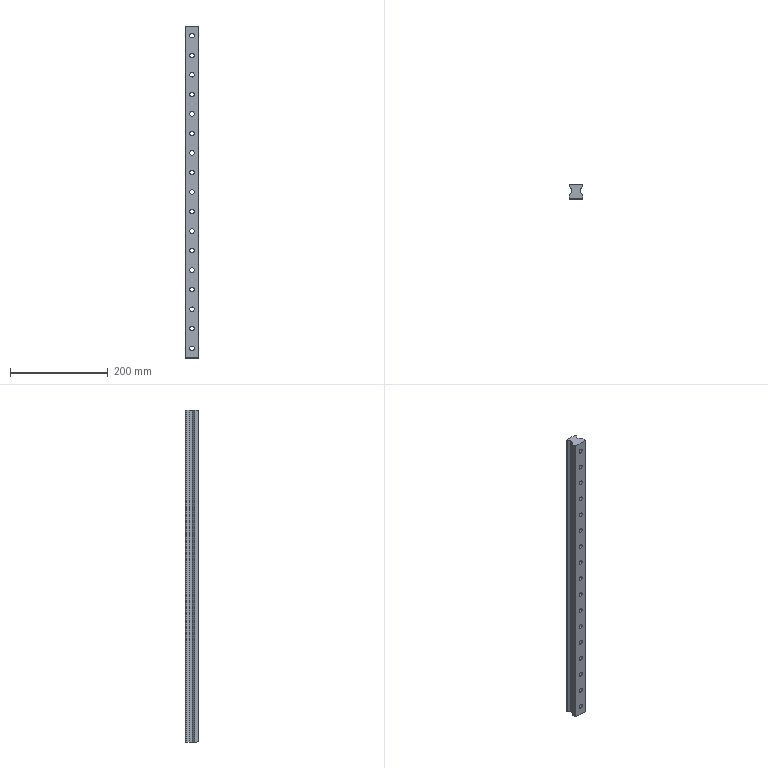Part | SolidWorks | features BaseBody 1 | 1 solid | 101 faces | box 28 x 28 x 680 mm | volume 401283 mm3 | cylinder 68 | plane 33 | commonest cylinder face diameters 9 x34 14 x34